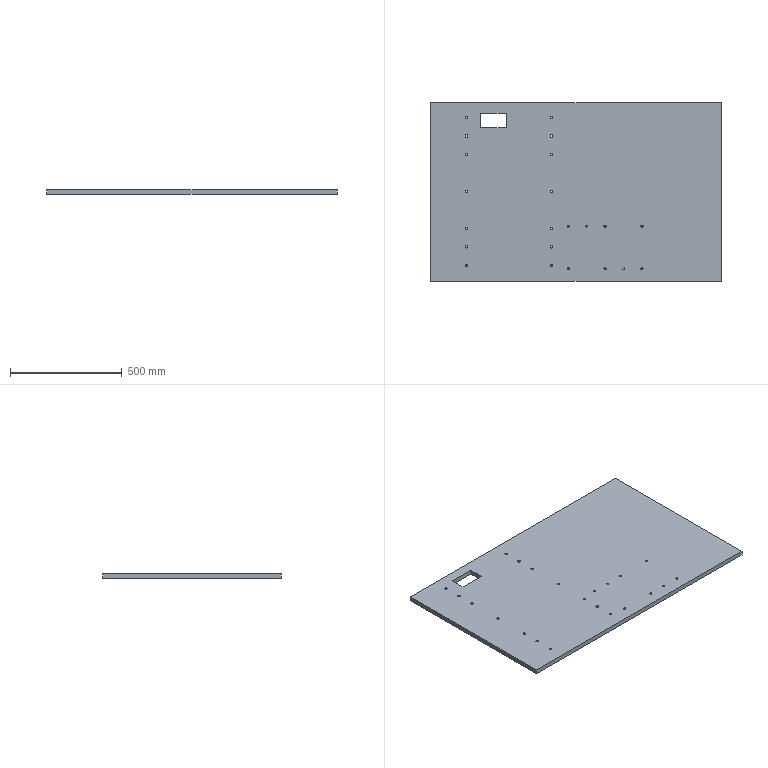Part | STEP file | Tube feed_id874_x_t | 1 solid | 64 faces | box 1300 x 800 x 21 mm | volume 21652093 mm3 | cone 32 | cylinder 22 | plane 10 | commonest cylinder face diameters 8.5 x16 12 x4 8 x2